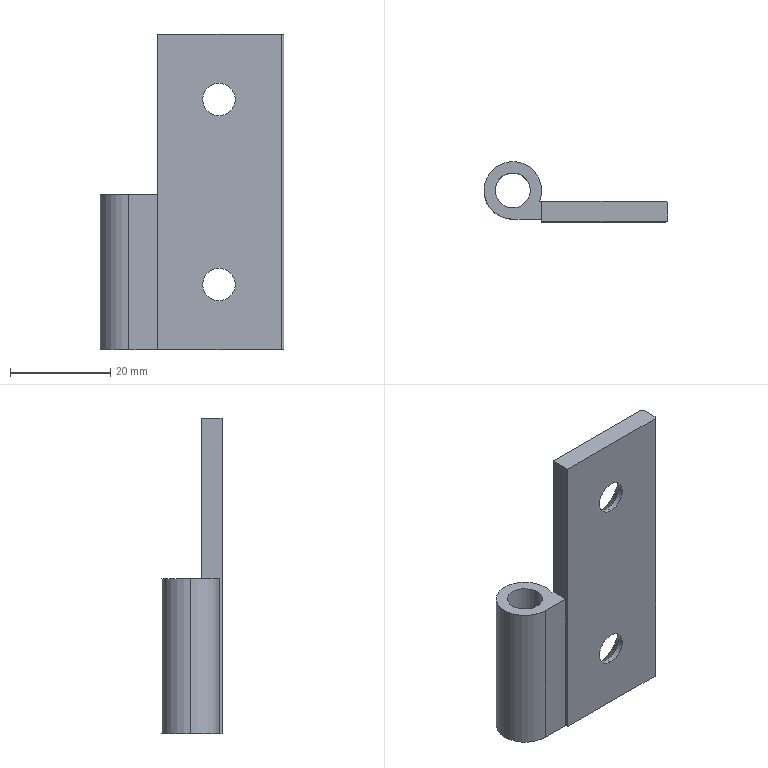Part | STEP file | _AKQ01怡合达合页2- | 1 solid | 23 faces | box 36.75 x 12.05 x 63 mm | volume 8240 mm3 | cylinder 11 | plane 8 | cone 4 | commonest cylinder face diameters 6.5 x4 11.5 x3 1 x2 7 x2
STEP:
#1=CARTESIAN_POINT('',(18.,0.,-15.25));
#2=VERTEX_POINT('',#1);
#3=CARTESIAN_POINT('',(18.,0.,-21.75));
#4=VERTEX_POINT('',#3);
#5=CARTESIAN_POINT('',(18.,0.,-18.5));
#6=DIRECTION('',(0.,-1.,0.));
#7=DIRECTION('',(0.,0.,1.));
#8=AXIS2_PLACEMENT_3D('',#5,#6,#7);
#9=CIRCLE('',#8,3.25);
#10=EDGE_CURVE('',#2,#4,#9,.T.);
#11=ORIENTED_EDGE('',*,*,#10,.T.);
#12=CARTESIAN_POINT('',(18.,1.1,-21.75));
#13=VERTEX_POINT('',#12);
#14=CARTESIAN_POINT('',(18.,0.,-21.75));
#15=DIRECTION('',(0.,1.,0.));
#16=VECTOR('',#15,1000.);
#17=LINE('',#14,#16);
#18=EDGE_CURVE('',#4,#13,#17,.T.);
#19=ORIENTED_EDGE('',*,*,#18,.T.);
#20=CARTESIAN_POINT('',(18.,1.1,-15.25));
#21=VERTEX_POINT('',#20);
#22=CARTESIAN_POINT('',(18.,1.1,-18.5));
#23=DIRECTION('',(0.,-1.,0.));
#24=DIRECTION('',(0.,0.,1.));
#25=AXIS2_PLACEMENT_3D('',#22,#23,#24);
#26=CIRCLE('',#25,3.25);
#27=EDGE_CURVE('',#21,#13,#26,.T.);
#28=ORIENTED_EDGE('',*,*,#27,.F.);
#29=CARTESIAN_POINT('',(18.,0.,-15.25));
#30=DIRECTION('',(0.,1.,0.));
#31=VECTOR('',#30,1000.);
#32=LINE('',#29,#31);
#33=EDGE_CURVE('',#2,#21,#32,.T.);
#34=ORIENTED_EDGE('',*,*,#33,.F.);
#35=EDGE_LOOP('',(#11,#19,#28,#34));
#36=FACE_OUTER_BOUND('',#35,.T.);
#37=CARTESIAN_POINT('',(18.,0.,-18.5));
#38=DIRECTION('',(0.,1.,0.));
#39=DIRECTION('',(0.,0.,1.));
#40=AXIS2_PLACEMENT_3D('',#37,#38,#39);
#41=CYLINDRICAL_SURFACE('',#40,3.25);
#42=ADVANCED_FACE('',(#36),#41,.F.);
#43=CARTESIAN_POINT('',(18.,0.,21.75));
#44=VERTEX_POINT('',#43);
#45=CARTESIAN_POINT('',(18.,0.,15.25));
#46=VERTEX_POINT('',#45);
#47=CARTESIAN_POINT('',(18.,0.,18.5));
#48=DIRECTION('',(0.,-1.,0.));
#49=DIRECTION('',(0.,0.,1.));
#50=AXIS2_PLACEMENT_3D('',#47,#48,#49);
#51=CIRCLE('',#50,3.25);
#52=EDGE_CURVE('',#44,#46,#51,.T.);
#53=ORIENTED_EDGE('',*,*,#52,.T.);
#54=CARTESIAN_POINT('',(18.,1.1,15.25));
#55=VERTEX_POINT('',#54);
#56=CARTESIAN_POINT('',(18.,0.,15.25));
#57=DIRECTION('',(0.,1.,0.));
#58=VECTOR('',#57,1000.);
#59=LINE('',#56,#58);
#60=EDGE_CURVE('',#46,#55,#59,.T.);
#61=ORIENTED_EDGE('',*,*,#60,.T.);
#62=CARTESIAN_POINT('',(18.,1.1,21.75));
#63=VERTEX_POINT('',#62);
#64=CARTESIAN_POINT('',(18.,1.1,18.5));
#65=DIRECTION('',(0.,-1.,0.));
#66=DIRECTION('',(0.,0.,1.));
#67=AXIS2_PLACEMENT_3D('',#64,#65,#66);
#68=CIRCLE('',#67,3.25);
#69=EDGE_CURVE('',#63,#55,#68,.T.);
#70=ORIENTED_EDGE('',*,*,#69,.F.);
#71=CARTESIAN_POINT('',(18.,0.,21.75));
#72=DIRECTION('',(0.,1.,0.));
#73=VECTOR('',#72,1000.);
#74=LINE('',#71,#73);
#75=EDGE_CURVE('',#44,#63,#74,.T.);
#76=ORIENTED_EDGE('',*,*,#75,.F.);
#77=EDGE_LOOP('',(#53,#61,#70,#76));
#78=FACE_OUTER_BOUND('',#77,.T.);
#79=CARTESIAN_POINT('',(18.,0.,18.5));
#80=DIRECTION('',(0.,1.,0.));
#81=DIRECTION('',(0.,0.,1.));
#82=AXIS2_PLACEMENT_3D('',#79,#80,#81);
#83=CYLINDRICAL_SURFACE('',#82,3.25);
#84=ADVANCED_FACE('',(#78),#83,.F.);
#85=CARTESIAN_POINT('',(5.75,6.3,-31.5));
#86=VERTEX_POINT('',#85);
#87=CARTESIAN_POINT('',(-5.75,6.3,-31.5));
#88=VERTEX_POINT('',#87);
#89=CARTESIAN_POINT('',(0.,6.3,-31.5));
#90=DIRECTION('',(0.,0.,1.));
#91=DIRECTION('',(1.,0.,0.));
#92=AXIS2_PLACEMENT_3D('',#89,#90,#91);
#93=CIRCLE('',#92,5.75);
#94=EDGE_CURVE('',#86,#88,#93,.T.);
#95=ORIENTED_EDGE('',*,*,#94,.T.);
#96=CARTESIAN_POINT('',(-5.75,6.3,-0.5));
#97=VERTEX_POINT('',#96);
#98=CARTESIAN_POINT('',(-5.75,6.3,31.5));
#99=DIRECTION('',(0.,0.,1.));
#100=VECTOR('',#99,1000.);
#101=LINE('',#98,#100);
#102=EDGE_CURVE('',#88,#97,#101,.T.);
#103=ORIENTED_EDGE('',*,*,#102,.T.);
#104=CARTESIAN_POINT('',(5.75,6.3,-0.5));
#105=VERTEX_POINT('',#104);
#106=CARTESIAN_POINT('',(0.,6.3,-0.5));
#107=DIRECTION('',(0.,0.,-1.));
#108=DIRECTION('',(1.,0.,0.));
#109=AXIS2_PLACEMENT_3D('',#106,#107,#108);
#110=CIRCLE('',#109,5.75);
#111=EDGE_CURVE('',#97,#105,#110,.T.);
#112=ORIENTED_EDGE('',*,*,#111,.T.);
#113=CARTESIAN_POINT('',(5.75,6.3,31.5));
#114=DIRECTION('',(0.,0.,1.));
#115=VECTOR('',#114,1000.);
#116=LINE('',#113,#115);
#117=EDGE_CURVE('',#86,#105,#116,.T.);
#118=ORIENTED_EDGE('',*,*,#117,.F.);
#119=EDGE_LOOP('',(#95,#103,#112,#118));
#120=FACE_OUTER_BOUND('',#119,.T.);
#121=CARTESIAN_POINT('',(0.,6.3,31.5));
#122=DIRECTION('',(0.,0.,1.));
#123=DIRECTION('',(1.,0.,0.));
#124=AXIS2_PLACEMENT_3D('',#121,#122,#123);
#125=CYLINDRICAL_SURFACE('',#124,5.75);
#126=ADVANCED_FACE('',(#120),#125,.T.);
#127=CARTESIAN_POINT('',(5.312,4.1,-31.5));
#128=VERTEX_POINT('',#127);
#129=CARTESIAN_POINT('',(0.,6.3,-31.5));
#130=DIRECTION('',(0.,0.,1.));
#131=DIRECTION('',(1.,0.,0.));
#132=AXIS2_PLACEMENT_3D('',#129,#130,#131);
#133=CIRCLE('',#132,5.75);
#134=EDGE_CURVE('',#128,#86,#133,.T.);
#135=ORIENTED_EDGE('',*,*,#134,.T.);
#136=ORIENTED_EDGE('',*,*,#117,.T.);
#137=CARTESIAN_POINT('',(5.312,4.1,-0.5));
#138=VERTEX_POINT('',#137);
#139=CARTESIAN_POINT('',(0.,6.3,-0.5));
#140=DIRECTION('',(0.,0.,-1.));
#141=DIRECTION('',(1.,0.,0.));
#142=AXIS2_PLACEMENT_3D('',#139,#140,#141);
#143=CIRCLE('',#142,5.75);
#144=EDGE_CURVE('',#105,#138,#143,.T.);
#145=ORIENTED_EDGE('',*,*,#144,.T.);
#146=CARTESIAN_POINT('',(5.312,4.1,31.5));
#147=DIRECTION('',(0.,0.,-1.));
#148=VECTOR('',#147,1000.);
#149=LINE('',#146,#148);
#150=EDGE_CURVE('',#138,#128,#149,.T.);
#151=ORIENTED_EDGE('',*,*,#150,.T.);
#152=EDGE_LOOP('',(#135,#136,#145,#151));
#153=FACE_OUTER_BOUND('',#152,.T.);
#154=CARTESIAN_POINT('',(0.,6.3,31.5));
#155=DIRECTION('',(0.,0.,1.));
#156=DIRECTION('',(1.,0.,0.));
#157=AXIS2_PLACEMENT_3D('',#154,#155,#156);
#158=CYLINDRICAL_SURFACE('',#157,5.75);
#159=ADVANCED_FACE('',(#153),#158,.T.);
#160=CARTESIAN_POINT('',(3.5,6.3,-31.5));
#161=VERTEX_POINT('',#160);
#162=CARTESIAN_POINT('',(-3.5,6.3,-31.5));
#163=VERTEX_POINT('',#162);
#164=CARTESIAN_POINT('',(0.,6.3,-31.5));
#165=DIRECTION('',(0.,0.,-1.));
#166=DIRECTION('',(1.,0.,0.));
#167=AXIS2_PLACEMENT_3D('',#164,#165,#166);
#168=CIRCLE('',#167,3.5);
#169=EDGE_CURVE('',#161,#163,#168,.T.);
#170=ORIENTED_EDGE('',*,*,#169,.T.);
#171=CARTESIAN_POINT('',(-3.5,6.3,-0.5));
#172=VERTEX_POINT('',#171);
#173=CARTESIAN_POINT('',(-3.5,6.3,31.5));
#174=DIRECTION('',(0.,0.,1.));
#175=VECTOR('',#174,1000.);
#176=LINE('',#173,#175);
#177=EDGE_CURVE('',#163,#172,#176,.T.);
#178=ORIENTED_EDGE('',*,*,#177,.T.);
#179=CARTESIAN_POINT('',(3.5,6.3,-0.5));
#180=VERTEX_POINT('',#179);
#181=CARTESIAN_POINT('',(0.,6.3,-0.5));
#182=DIRECTION('',(0.,0.,-1.));
#183=DIRECTION('',(1.,0.,0.));
#184=AXIS2_PLACEMENT_3D('',#181,#182,#183);
#185=CIRCLE('',#184,3.5);
#186=EDGE_CURVE('',#180,#172,#185,.T.);
#187=ORIENTED_EDGE('',*,*,#186,.F.);
#188=CARTESIAN_POINT('',(3.5,6.3,31.5));
#189=DIRECTION('',(0.,0.,1.));
#190=VECTOR('',#189,1000.);
#191=LINE('',#188,#190);
#192=EDGE_CURVE('',#161,#180,#191,.T.);
#193=ORIENTED_EDGE('',*,*,#192,.F.);
#194=EDGE_LOOP('',(#170,#178,#187,#193));
#195=FACE_OUTER_BOUND('',#194,.T.);
#196=CARTESIAN_POINT('',(0.,6.3,31.5));
#197=DIRECTION('',(0.,0.,1.));
#198=DIRECTION('',(1.,0.,0.));
#199=AXIS2_PLACEMENT_3D('',#196,#197,#198);
#200=CYLINDRICAL_SURFACE('',#199,3.5);
#201=ADVANCED_FACE('',(#195),#200,.F.);
#202=ORIENTED_EDGE('',*,*,#27,.T.);
#203=CARTESIAN_POINT('',(18.,4.1,-24.75));
#204=VERTEX_POINT('',#203);
#205=CARTESIAN_POINT('',(18.,4.1,-24.75));
#206=DIRECTION('',(0.,0.7071,-0.7071));
#207=VECTOR('',#206,1000.);
#208=LINE('',#205,#207);
#209=EDGE_CURVE('',#13,#204,#208,.T.);
#210=ORIENTED_EDGE('',*,*,#209,.T.);
#211=CARTESIAN_POINT('',(18.,4.1,-12.25));
#212=VERTEX_POINT('',#211);
#213=CARTESIAN_POINT('',(18.,4.1,-18.5));
#214=DIRECTION('',(0.,1.,0.));
#215=DIRECTION('',(0.,0.,1.));
#216=AXIS2_PLACEMENT_3D('',#213,#214,#215);
#217=CIRCLE('',#216,6.25);
#218=EDGE_CURVE('',#204,#212,#217,.T.);
#219=ORIENTED_EDGE('',*,*,#218,.T.);
#220=CARTESIAN_POINT('',(18.,4.1,-12.25));
#221=DIRECTION('',(0.,0.7071,0.7071));
#222=VECTOR('',#221,1000.);
#223=LINE('',#220,#222);
#224=EDGE_CURVE('',#21,#212,#223,.T.);
#225=ORIENTED_EDGE('',*,*,#224,.F.);
#226=EDGE_LOOP('',(#202,#210,#219,#225));
#227=FACE_OUTER_BOUND('',#226,.T.);
#228=CARTESIAN_POINT('',(18.,4.1,-18.5));
#229=DIRECTION('',(0.,1.,0.));
#230=DIRECTION('',(0.,0.,1.));
#231=AXIS2_PLACEMENT_3D('',#228,#229,#230);
#232=CONICAL_SURFACE('',#231,6.25,0.7854);
#233=ADVANCED_FACE('',(#227),#232,.F.);
#234=ORIENTED_EDGE('',*,*,#69,.T.);
#235=CARTESIAN_POINT('',(18.,4.1,12.25));
#236=VERTEX_POINT('',#235);
#237=CARTESIAN_POINT('',(18.,4.1,12.25));
#238=DIRECTION('',(0.,0.7071,-0.7071));
#239=VECTOR('',#238,1000.);
#240=LINE('',#237,#239);
#241=EDGE_CURVE('',#55,#236,#240,.T.);
#242=ORIENTED_EDGE('',*,*,#241,.T.);
#243=CARTESIAN_POINT('',(18.,4.1,24.75));
#244=VERTEX_POINT('',#243);
#245=CARTESIAN_POINT('',(18.,4.1,18.5));
#246=DIRECTION('',(0.,1.,0.));
#247=DIRECTION('',(0.,0.,1.));
#248=AXIS2_PLACEMENT_3D('',#245,#246,#247);
#249=CIRCLE('',#248,6.25);
#250=EDGE_CURVE('',#236,#244,#249,.T.);
#251=ORIENTED_EDGE('',*,*,#250,.T.);
#252=CARTESIAN_POINT('',(18.,4.1,24.75));
#253=DIRECTION('',(0.,0.7071,0.7071));
#254=VECTOR('',#253,1000.);
#255=LINE('',#252,#254);
#256=EDGE_CURVE('',#63,#244,#255,.T.);
#257=ORIENTED_EDGE('',*,*,#256,.F.);
#258=EDGE_LOOP('',(#234,#242,#251,#257));
#259=FACE_OUTER_BOUND('',#258,.T.);
#260=CARTESIAN_POINT('',(18.,4.1,18.5));
#261=DIRECTION('',(0.,1.,0.));
#262=DIRECTION('',(0.,0.,1.));
#263=AXIS2_PLACEMENT_3D('',#260,#261,#262);
#264=CONICAL_SURFACE('',#263,6.25,0.7854);
#265=ADVANCED_FACE('',(#259),#264,.F.);
#266=CARTESIAN_POINT('',(30.5,0.,31.5));
#267=VERTEX_POINT('',#266);
#268=CARTESIAN_POINT('',(30.5,0.,-31.5));
#269=VERTEX_POINT('',#268);
#270=CARTESIAN_POINT('',(30.5,0.,31.5));
#271=DIRECTION('',(0.,0.,-1.));
#272=VECTOR('',#271,1000.);
#273=LINE('',#270,#272);
#274=EDGE_CURVE('',#267,#269,#273,.T.);
#275=ORIENTED_EDGE('',*,*,#274,.F.);
#276=CARTESIAN_POINT('',(5.75,0.,31.5));
#277=VERTEX_POINT('',#276);
#278=CARTESIAN_POINT('',(5.75,0.,31.5));
#279=DIRECTION('',(1.,0.,0.));
#280=VECTOR('',#279,1000.);
#281=LINE('',#278,#280);
#282=EDGE_CURVE('',#277,#267,#281,.T.);
#283=ORIENTED_EDGE('',*,*,#282,.F.);
#284=CARTESIAN_POINT('',(5.75,0.,-31.5));
#285=VERTEX_POINT('',#284);
#286=CARTESIAN_POINT('',(5.75,0.,31.5));
#287=DIRECTION('',(0.,0.,1.));
#288=VECTOR('',#287,1000.);
#289=LINE('',#286,#288);
#290=EDGE_CURVE('',#285,#277,#289,.T.);
#291=ORIENTED_EDGE('',*,*,#290,.F.);
#292=CARTESIAN_POINT('',(5.75,0.,-31.5));
#293=DIRECTION('',(-1.,0.,0.));
#294=VECTOR('',#293,1000.);
#295=LINE('',#292,#294);
#296=EDGE_CURVE('',#269,#285,#295,.T.);
#297=ORIENTED_EDGE('',*,*,#296,.F.);
#298=EDGE_LOOP('',(#275,#283,#291,#297));
#299=FACE_OUTER_BOUND('',#298,.T.);
#300=ORIENTED_EDGE('',*,*,#10,.F.);
#301=CARTESIAN_POINT('',(18.,0.,-18.5));
#302=DIRECTION('',(0.,-1.,0.));
#303=DIRECTION('',(0.,0.,1.));
#304=AXIS2_PLACEMENT_3D('',#301,#302,#303);
#305=CIRCLE('',#304,3.25);
#306=EDGE_CURVE('',#4,#2,#305,.T.);
#307=ORIENTED_EDGE('',*,*,#306,.F.);
#308=EDGE_LOOP('',(#300,#307));
#309=FACE_BOUND('',#308,.T.);
#310=ORIENTED_EDGE('',*,*,#52,.F.);
#311=CARTESIAN_POINT('',(18.,0.,18.5));
#312=DIRECTION('',(0.,-1.,0.));
#313=DIRECTION('',(0.,0.,1.));
#314=AXIS2_PLACEMENT_3D('',#311,#312,#313);
#315=CIRCLE('',#314,3.25);
#316=EDGE_CURVE('',#46,#44,#315,.T.);
#317=ORIENTED_EDGE('',*,*,#316,.F.);
#318=EDGE_LOOP('',(#310,#317));
#319=FACE_BOUND('',#318,.T.);
#320=CARTESIAN_POINT('',(5.75,0.,31.5));
#321=DIRECTION('',(0.,1.,0.));
#322=DIRECTION('',(0.,0.,1.));
#323=AXIS2_PLACEMENT_3D('',#320,#321,#322);
#324=PLANE('',#323);
#325=ADVANCED_FACE('',(#299,#309,#319),#324,.F.);
#326=CARTESIAN_POINT('',(31.,3.6,-31.5));
#327=VERTEX_POINT('',#326);
#328=CARTESIAN_POINT('',(30.5,4.1,-31.5));
#329=VERTEX_POINT('',#328);
#330=CARTESIAN_POINT('',(30.5,3.6,-31.5));
#331=DIRECTION('',(0.,0.,1.));
#332=DIRECTION('',(1.,0.,0.));
#333=AXIS2_PLACEMENT_3D('',#330,#331,#332);
#334=CIRCLE('',#333,0.5);
#335=EDGE_CURVE('',#327,#329,#334,.T.);
#336=ORIENTED_EDGE('',*,*,#335,.F.);
#337=CARTESIAN_POINT('',(31.,0.5,-31.5));
#338=VERTEX_POINT('',#337);
#339=CARTESIAN_POINT('',(31.,6.3,-31.5));
#340=DIRECTION('',(0.,1.,0.));
#341=VECTOR('',#340,1000.);
#342=LINE('',#339,#341);
#343=EDGE_CURVE('',#338,#327,#342,.T.);
#344=ORIENTED_EDGE('',*,*,#343,.F.);
#345=CARTESIAN_POINT('',(30.5,0.5,-31.5));
#346=DIRECTION('',(0.,0.,1.));
#347=DIRECTION('',(1.,0.,0.));
#348=AXIS2_PLACEMENT_3D('',#345,#346,#347);
#349=CIRCLE('',#348,0.5);
#350=EDGE_CURVE('',#269,#338,#349,.T.);
#351=ORIENTED_EDGE('',*,*,#350,.F.);
#352=ORIENTED_EDGE('',*,*,#296,.T.);
#353=CARTESIAN_POINT('',(5.75,0.55,-31.5));
#354=VERTEX_POINT('',#353);
#355=CARTESIAN_POINT('',(5.75,6.3,-31.5));
#356=DIRECTION('',(0.,-1.,0.));
#357=VECTOR('',#356,1000.);
#358=LINE('',#355,#357);
#359=EDGE_CURVE('',#354,#285,#358,.T.);
#360=ORIENTED_EDGE('',*,*,#359,.F.);
#361=CARTESIAN_POINT('',(0.,0.55,-31.5));
#362=VERTEX_POINT('',#361);
#363=CARTESIAN_POINT('',(0.,0.55,-31.5));
#364=DIRECTION('',(1.,0.,0.));
#365=VECTOR('',#364,1000.);
#366=LINE('',#363,#365);
#367=EDGE_CURVE('',#362,#354,#366,.T.);
#368=ORIENTED_EDGE('',*,*,#367,.F.);
#369=CARTESIAN_POINT('',(0.,6.3,-31.5));
#370=DIRECTION('',(0.,0.,1.));
#371=DIRECTION('',(1.,0.,0.));
#372=AXIS2_PLACEMENT_3D('',#369,#370,#371);
#373=CIRCLE('',#372,5.75);
#374=EDGE_CURVE('',#88,#362,#373,.T.);
#375=ORIENTED_EDGE('',*,*,#374,.F.);
#376=ORIENTED_EDGE('',*,*,#94,.F.);
#377=ORIENTED_EDGE('',*,*,#134,.F.);
#378=CARTESIAN_POINT('',(0.,4.1,-31.5));
#379=DIRECTION('',(-1.,0.,0.));
#380=VECTOR('',#379,1000.);
#381=LINE('',#378,#380);
#382=EDGE_CURVE('',#329,#128,#381,.T.);
#383=ORIENTED_EDGE('',*,*,#382,.F.);
#384=EDGE_LOOP('',(#336,#344,#351,#352,#360,#368,#375,#376,#377,#383));
#385=FACE_OUTER_BOUND('',#384,.T.);
#386=ORIENTED_EDGE('',*,*,#169,.F.);
#387=CARTESIAN_POINT('',(0.,6.3,-31.5));
#388=DIRECTION('',(0.,0.,-1.));
#389=DIRECTION('',(1.,0.,0.));
#390=AXIS2_PLACEMENT_3D('',#387,#388,#389);
#391=CIRCLE('',#390,3.5);
#392=EDGE_CURVE('',#163,#161,#391,.T.);
#393=ORIENTED_EDGE('',*,*,#392,.F.);
#394=EDGE_LOOP('',(#386,#393));
#395=FACE_BOUND('',#394,.T.);
#396=CARTESIAN_POINT('',(0.,6.3,-31.5));
#397=DIRECTION('',(0.,0.,1.));
#398=DIRECTION('',(1.,0.,0.));
#399=AXIS2_PLACEMENT_3D('',#396,#397,#398);
#400=PLANE('',#399);
#401=ADVANCED_FACE('',(#385,#395),#400,.F.);
#402=CARTESIAN_POINT('',(31.,0.5,31.5));
#403=VERTEX_POINT('',#402);
#404=CARTESIAN_POINT('',(30.5,0.5,31.5));
#405=DIRECTION('',(0.,0.,-1.));
#406=DIRECTION('',(1.,0.,0.));
#407=AXIS2_PLACEMENT_3D('',#404,#405,#406);
#408=CIRCLE('',#407,0.5);
#409=EDGE_CURVE('',#403,#267,#408,.T.);
#410=ORIENTED_EDGE('',*,*,#409,.T.);
#411=ORIENTED_EDGE('',*,*,#274,.T.);
#412=ORIENTED_EDGE('',*,*,#350,.T.);
#413=CARTESIAN_POINT('',(31.,0.5,31.5));
#414=DIRECTION('',(0.,0.,1.));
#415=VECTOR('',#414,1000.);
#416=LINE('',#413,#415);
#417=EDGE_CURVE('',#338,#403,#416,.T.);
#418=ORIENTED_EDGE('',*,*,#417,.T.);
#419=EDGE_LOOP('',(#410,#411,#412,#418));
#420=FACE_OUTER_BOUND('',#419,.T.);
#421=CARTESIAN_POINT('',(30.5,0.5,31.5));
#422=DIRECTION('',(0.,0.,1.));
#423=DIRECTION('',(1.,0.,0.));
#424=AXIS2_PLACEMENT_3D('',#421,#422,#423);
#425=CYLINDRICAL_SURFACE('',#424,0.5);
#426=ADVANCED_FACE('',(#420),#425,.T.);
#427=CARTESIAN_POINT('',(31.,3.6,31.5));
#428=VERTEX_POINT('',#427);
#429=CARTESIAN_POINT('',(31.,6.3,31.5));
#430=DIRECTION('',(0.,1.,0.));
#431=VECTOR('',#430,1000.);
#432=LINE('',#429,#431);
#433=EDGE_CURVE('',#403,#428,#432,.T.);
#434=ORIENTED_EDGE('',*,*,#433,.T.);
#435=CARTESIAN_POINT('',(30.5,4.1,31.5));
#436=VERTEX_POINT('',#435);
#437=CARTESIAN_POINT('',(30.5,3.6,31.5));
#438=DIRECTION('',(0.,0.,-1.));
#439=DIRECTION('',(1.,0.,0.));
#440=AXIS2_PLACEMENT_3D('',#437,#438,#439);
#441=CIRCLE('',#440,0.5);
#442=EDGE_CURVE('',#436,#428,#441,.T.);
#443=ORIENTED_EDGE('',*,*,#442,.F.);
#444=CARTESIAN_POINT('',(5.75,4.1,31.5));
#445=VERTEX_POINT('',#444);
#446=CARTESIAN_POINT('',(0.,4.1,31.5));
#447=DIRECTION('',(-1.,0.,0.));
#448=VECTOR('',#447,1000.);
#449=LINE('',#446,#448);
#450=EDGE_CURVE('',#436,#445,#449,.T.);
#451=ORIENTED_EDGE('',*,*,#450,.T.);
#452=CARTESIAN_POINT('',(5.75,6.3,31.5));
#453=DIRECTION('',(0.,-1.,0.));
#454=VECTOR('',#453,1000.);
#455=LINE('',#452,#454);
#456=EDGE_CURVE('',#445,#277,#455,.T.);
#457=ORIENTED_EDGE('',*,*,#456,.T.);
#458=ORIENTED_EDGE('',*,*,#282,.T.);
#459=ORIENTED_EDGE('',*,*,#409,.F.);
#460=EDGE_LOOP('',(#434,#443,#451,#457,#458,#459));
#461=FACE_OUTER_BOUND('',#460,.T.);
#462=CARTESIAN_POINT('',(0.,6.3,31.5));
#463=DIRECTION('',(0.,0.,1.));
#464=DIRECTION('',(1.,0.,0.));
#465=AXIS2_PLACEMENT_3D('',#462,#463,#464);
#466=PLANE('',#465);
#467=ADVANCED_FACE('',(#461),#466,.T.);
#468=CARTESIAN_POINT('',(5.75,4.1,-0.5));
#469=VERTEX_POINT('',#468);
#470=CARTESIAN_POINT('',(5.75,4.1,31.5));
#471=DIRECTION('',(0.,0.,1.));
#472=VECTOR('',#471,1000.);
#473=LINE('',#470,#472);
#474=EDGE_CURVE('',#469,#445,#473,.T.);
#475=ORIENTED_EDGE('',*,*,#474,.F.);
#476=CARTESIAN_POINT('',(5.75,0.55,-0.5));
#477=VERTEX_POINT('',#476);
#478=CARTESIAN_POINT('',(5.75,0.55,-0.5));
#479=DIRECTION('',(0.,1.,0.));
#480=VECTOR('',#479,1000.);
#481=LINE('',#478,#480);
#482=EDGE_CURVE('',#477,#469,#481,.T.);
#483=ORIENTED_EDGE('',*,*,#482,.F.);
#484=CARTESIAN_POINT('',(5.75,0.55,31.5));
#485=DIRECTION('',(0.,0.,1.));
#486=VECTOR('',#485,1000.);
#487=LINE('',#484,#486);
#488=EDGE_CURVE('',#354,#477,#487,.T.);
#489=ORIENTED_EDGE('',*,*,#488,.F.);
#490=ORIENTED_EDGE('',*,*,#359,.T.);
#491=ORIENTED_EDGE('',*,*,#290,.T.);
#492=ORIENTED_EDGE('',*,*,#456,.F.);
#493=EDGE_LOOP('',(#475,#483,#489,#490,#491,#492));
#494=FACE_OUTER_BOUND('',#493,.T.);
#495=CARTESIAN_POINT('',(5.75,0.55,31.5));
#496=DIRECTION('',(1.,0.,0.));
#497=DIRECTION('',(0.,1.,0.));
#498=AXIS2_PLACEMENT_3D('',#495,#496,#497);
#499=PLANE('',#498);
#500=ADVANCED_FACE('',(#494),#499,.F.);
#501=ORIENTED_EDGE('',*,*,#18,.F.);
#502=ORIENTED_EDGE('',*,*,#306,.T.);
#503=ORIENTED_EDGE('',*,*,#33,.T.);
#504=CARTESIAN_POINT('',(18.,1.1,-18.5));
#505=DIRECTION('',(0.,-1.,0.));
#506=DIRECTION('',(0.,0.,1.));
#507=AXIS2_PLACEMENT_3D('',#504,#505,#506);
#508=CIRCLE('',#507,3.25);
#509=EDGE_CURVE('',#13,#21,#508,.T.);
#510=ORIENTED_EDGE('',*,*,#509,.F.);
#511=EDGE_LOOP('',(#501,#502,#503,#510));
#512=FACE_OUTER_BOUND('',#511,.T.);
#513=CARTESIAN_POINT('',(18.,0.,-18.5));
#514=DIRECTION('',(0.,1.,0.));
#515=DIRECTION('',(0.,0.,1.));
#516=AXIS2_PLACEMENT_3D('',#513,#514,#515);
#517=CYLINDRICAL_SURFACE('',#516,3.25);
#518=ADVANCED_FACE('',(#512),#517,.F.);
#519=ORIENTED_EDGE('',*,*,#60,.F.);
#520=ORIENTED_EDGE('',*,*,#316,.T.);
#521=ORIENTED_EDGE('',*,*,#75,.T.);
#522=CARTESIAN_POINT('',(18.,1.1,18.5));
#523=DIRECTION('',(0.,-1.,0.));
#524=DIRECTION('',(0.,0.,1.));
#525=AXIS2_PLACEMENT_3D('',#522,#523,#524);
#526=CIRCLE('',#525,3.25);
#527=EDGE_CURVE('',#55,#63,#526,.T.);
#528=ORIENTED_EDGE('',*,*,#527,.F.);
#529=EDGE_LOOP('',(#519,#520,#521,#528));
#530=FACE_OUTER_BOUND('',#529,.T.);
#531=CARTESIAN_POINT('',(18.,0.,18.5));
#532=DIRECTION('',(0.,1.,0.));
#533=DIRECTION('',(0.,0.,1.));
#534=AXIS2_PLACEMENT_3D('',#531,#532,#533);
#535=CYLINDRICAL_SURFACE('',#534,3.25);
#536=ADVANCED_FACE('',(#530),#535,.F.);
#537=ORIENTED_EDGE('',*,*,#450,.F.);
#538=CARTESIAN_POINT('',(30.5,4.1,31.5));
#539=DIRECTION('',(0.,0.,1.));
#540=VECTOR('',#539,1000.);
#541=LINE('',#538,#540);
#542=EDGE_CURVE('',#329,#436,#541,.T.);
#543=ORIENTED_EDGE('',*,*,#542,.F.);
#544=ORIENTED_EDGE('',*,*,#382,.T.);
#545=ORIENTED_EDGE('',*,*,#150,.F.);
#546=CARTESIAN_POINT('',(30.5,4.1,-0.5));
#547=DIRECTION('',(-1.,0.,0.));
#548=VECTOR('',#547,1000.);
#549=LINE('',#546,#548);
#550=EDGE_CURVE('',#469,#138,#549,.T.);
#551=ORIENTED_EDGE('',*,*,#550,.F.);
#552=ORIENTED_EDGE('',*,*,#474,.T.);
#553=EDGE_LOOP('',(#537,#543,#544,#545,#551,#552));
#554=FACE_OUTER_BOUND('',#553,.T.);
#555=CARTESIAN_POINT('',(18.,4.1,-18.5));
#556=DIRECTION('',(0.,1.,0.));
#557=DIRECTION('',(0.,0.,1.));
#558=AXIS2_PLACEMENT_3D('',#555,#556,#557);
#559=CIRCLE('',#558,6.25);
#560=EDGE_CURVE('',#212,#204,#559,.T.);
#561=ORIENTED_EDGE('',*,*,#560,.F.);
#562=ORIENTED_EDGE('',*,*,#218,.F.);
#563=EDGE_LOOP('',(#561,#562));
#564=FACE_BOUND('',#563,.T.);
#565=CARTESIAN_POINT('',(18.,4.1,18.5));
#566=DIRECTION('',(0.,1.,0.));
#567=DIRECTION('',(0.,0.,1.));
#568=AXIS2_PLACEMENT_3D('',#565,#566,#567);
#569=CIRCLE('',#568,6.25);
#570=EDGE_CURVE('',#244,#236,#569,.T.);
#571=ORIENTED_EDGE('',*,*,#570,.F.);
#572=ORIENTED_EDGE('',*,*,#250,.F.);
#573=EDGE_LOOP('',(#571,#572));
#574=FACE_BOUND('',#573,.T.);
#575=CARTESIAN_POINT('',(30.5,4.1,31.5));
#576=DIRECTION('',(0.,-1.,0.));
#577=DIRECTION('',(0.,0.,-1.));
#578=AXIS2_PLACEMENT_3D('',#575,#576,#577);
#579=PLANE('',#578);
#580=ADVANCED_FACE('',(#554,#564,#574),#579,.F.);
#581=CARTESIAN_POINT('',(31.,3.6,31.5));
#582=DIRECTION('',(0.,0.,-1.));
#583=VECTOR('',#582,1000.);
#584=LINE('',#581,#583);
#585=EDGE_CURVE('',#428,#327,#584,.T.);
#586=ORIENTED_EDGE('',*,*,#585,.F.);
#587=ORIENTED_EDGE('',*,*,#433,.F.);
#588=ORIENTED_EDGE('',*,*,#417,.F.);
#589=ORIENTED_EDGE('',*,*,#343,.T.);
#590=EDGE_LOOP('',(#586,#587,#588,#589));
#591=FACE_OUTER_BOUND('',#590,.T.);
#592=CARTESIAN_POINT('',(31.,0.5,31.5));
#593=DIRECTION('',(-1.,0.,0.));
#594=DIRECTION('',(0.,0.,1.));
#595=AXIS2_PLACEMENT_3D('',#592,#593,#594);
#596=PLANE('',#595);
#597=ADVANCED_FACE('',(#591),#596,.F.);
#598=CARTESIAN_POINT('',(0.,0.55,-0.5));
#599=VERTEX_POINT('',#598);
#600=CARTESIAN_POINT('',(0.,0.55,31.5));
#601=DIRECTION('',(0.,0.,1.));
#602=VECTOR('',#601,1000.);
#603=LINE('',#600,#602);
#604=EDGE_CURVE('',#362,#599,#603,.T.);
#605=ORIENTED_EDGE('',*,*,#604,.F.);
#606=ORIENTED_EDGE('',*,*,#367,.T.);
#607=ORIENTED_EDGE('',*,*,#488,.T.);
#608=CARTESIAN_POINT('',(0.,0.55,-0.5));
#609=DIRECTION('',(1.,0.,0.));
#610=VECTOR('',#609,1000.);
#611=LINE('',#608,#610);
#612=EDGE_CURVE('',#599,#477,#611,.T.);
#613=ORIENTED_EDGE('',*,*,#612,.F.);
#614=EDGE_LOOP('',(#605,#606,#607,#613));
#615=FACE_OUTER_BOUND('',#614,.T.);
#616=CARTESIAN_POINT('',(0.,0.55,31.5));
#617=DIRECTION('',(0.,1.,0.));
#618=DIRECTION('',(0.,0.,1.));
#619=AXIS2_PLACEMENT_3D('',#616,#617,#618);
#620=PLANE('',#619);
#621=ADVANCED_FACE('',(#615),#620,.F.);
#622=ORIENTED_EDGE('',*,*,#102,.F.);
#623=ORIENTED_EDGE('',*,*,#374,.T.);
#624=ORIENTED_EDGE('',*,*,#604,.T.);
#625=CARTESIAN_POINT('',(0.,6.3,-0.5));
#626=DIRECTION('',(0.,0.,-1.));
#627=DIRECTION('',(1.,0.,0.));
#628=AXIS2_PLACEMENT_3D('',#625,#626,#627);
#629=CIRCLE('',#628,5.75);
#630=EDGE_CURVE('',#599,#97,#629,.T.);
#631=ORIENTED_EDGE('',*,*,#630,.T.);
#632=EDGE_LOOP('',(#622,#623,#624,#631));
#633=FACE_OUTER_BOUND('',#632,.T.);
#634=CARTESIAN_POINT('',(0.,6.3,31.5));
#635=DIRECTION('',(0.,0.,1.));
#636=DIRECTION('',(1.,0.,0.));
#637=AXIS2_PLACEMENT_3D('',#634,#635,#636);
#638=CYLINDRICAL_SURFACE('',#637,5.75);
#639=ADVANCED_FACE('',(#633),#638,.T.);
#640=ORIENTED_EDGE('',*,*,#177,.F.);
#641=ORIENTED_EDGE('',*,*,#392,.T.);
#642=ORIENTED_EDGE('',*,*,#192,.T.);
#643=CARTESIAN_POINT('',(0.,6.3,-0.5));
#644=DIRECTION('',(0.,0.,-1.));
#645=DIRECTION('',(1.,0.,0.));
#646=AXIS2_PLACEMENT_3D('',#643,#644,#645);
#647=CIRCLE('',#646,3.5);
#648=EDGE_CURVE('',#172,#180,#647,.T.);
#649=ORIENTED_EDGE('',*,*,#648,.F.);
#650=EDGE_LOOP('',(#640,#641,#642,#649));
#651=FACE_OUTER_BOUND('',#650,.T.);
#652=CARTESIAN_POINT('',(0.,6.3,31.5));
#653=DIRECTION('',(0.,0.,1.));
#654=DIRECTION('',(1.,0.,0.));
#655=AXIS2_PLACEMENT_3D('',#652,#653,#654);
#656=CYLINDRICAL_SURFACE('',#655,3.5);
#657=ADVANCED_FACE('',(#651),#656,.F.);
#658=ORIENTED_EDGE('',*,*,#612,.T.);
#659=ORIENTED_EDGE('',*,*,#482,.T.);
#660=ORIENTED_EDGE('',*,*,#550,.T.);
#661=ORIENTED_EDGE('',*,*,#144,.F.);
#662=ORIENTED_EDGE('',*,*,#111,.F.);
#663=ORIENTED_EDGE('',*,*,#630,.F.);
#664=EDGE_LOOP('',(#658,#659,#660,#661,#662,#663));
#665=FACE_OUTER_BOUND('',#664,.T.);
#666=ORIENTED_EDGE('',*,*,#186,.T.);
#667=ORIENTED_EDGE('',*,*,#648,.T.);
#668=EDGE_LOOP('',(#666,#667));
#669=FACE_BOUND('',#668,.T.);
#670=CARTESIAN_POINT('',(5.75,25.4,-0.5));
#671=DIRECTION('',(0.,0.,1.));
#672=DIRECTION('',(1.,0.,0.));
#673=AXIS2_PLACEMENT_3D('',#670,#671,#672);
#674=PLANE('',#673);
#675=ADVANCED_FACE('',(#665,#669),#674,.T.);
#676=ORIENTED_EDGE('',*,*,#209,.F.);
#677=ORIENTED_EDGE('',*,*,#509,.T.);
#678=ORIENTED_EDGE('',*,*,#224,.T.);
#679=ORIENTED_EDGE('',*,*,#560,.T.);
#680=EDGE_LOOP('',(#676,#677,#678,#679));
#681=FACE_OUTER_BOUND('',#680,.T.);
#682=CARTESIAN_POINT('',(18.,4.1,-18.5));
#683=DIRECTION('',(0.,1.,0.));
#684=DIRECTION('',(0.,0.,1.));
#685=AXIS2_PLACEMENT_3D('',#682,#683,#684);
#686=CONICAL_SURFACE('',#685,6.25,0.7854);
#687=ADVANCED_FACE('',(#681),#686,.F.);
#688=ORIENTED_EDGE('',*,*,#241,.F.);
#689=ORIENTED_EDGE('',*,*,#527,.T.);
#690=ORIENTED_EDGE('',*,*,#256,.T.);
#691=ORIENTED_EDGE('',*,*,#570,.T.);
#692=EDGE_LOOP('',(#688,#689,#690,#691));
#693=FACE_OUTER_BOUND('',#692,.T.);
#694=CARTESIAN_POINT('',(18.,4.1,18.5));
#695=DIRECTION('',(0.,1.,0.));
#696=DIRECTION('',(0.,0.,1.));
#697=AXIS2_PLACEMENT_3D('',#694,#695,#696);
#698=CONICAL_SURFACE('',#697,6.25,0.7854);
#699=ADVANCED_FACE('',(#693),#698,.F.);
#700=ORIENTED_EDGE('',*,*,#442,.T.);
#701=ORIENTED_EDGE('',*,*,#585,.T.);
#702=ORIENTED_EDGE('',*,*,#335,.T.);
#703=ORIENTED_EDGE('',*,*,#542,.T.);
#704=EDGE_LOOP('',(#700,#701,#702,#703));
#705=FACE_OUTER_BOUND('',#704,.T.);
#706=CARTESIAN_POINT('',(30.5,3.6,31.5));
#707=DIRECTION('',(0.,0.,1.));
#708=DIRECTION('',(1.,0.,0.));
#709=AXIS2_PLACEMENT_3D('',#706,#707,#708);
#710=CYLINDRICAL_SURFACE('',#709,0.5);
#711=ADVANCED_FACE('',(#705),#710,.T.);
#712=CLOSED_SHELL('',(#42,#84,#126,#159,#201,#233,#265,#325,#401,#426,#467,#500,#518,#536,#580,#597,#621,#639,#657,#675,#687,#699,#711));
#713=MANIFOLD_SOLID_BREP('',#712);
#714=CARTESIAN_POINT('',(0.,0.,0.));
#715=DIRECTION('',(0.,0.,1.));
#716=DIRECTION('',(1.,0.,0.));
#717=AXIS2_PLACEMENT_3D('',#714,#715,#716);
#718=(LENGTH_UNIT()NAMED_UNIT(*)SI_UNIT(.MILLI.,.METRE.));
#719=UNCERTAINTY_MEASURE_WITH_UNIT(LENGTH_MEASURE(0.00001),#718,'','');
#720=(NAMED_UNIT(*)PLANE_ANGLE_UNIT()SI_UNIT($,.RADIAN.));
#721=(NAMED_UNIT(*)SI_UNIT($,.STERADIAN.)SOLID_ANGLE_UNIT());
#722=(GEOMETRIC_REPRESENTATION_CONTEXT(3)GLOBAL_UNCERTAINTY_ASSIGNED_CONTEXT((#719))GLOBAL_UNIT_ASSIGNED_CONTEXT((#718,#720,#721))REPRESENTATION_CONTEXT('',''));
#723=ADVANCED_BREP_SHAPE_REPRESENTATION('',(#713,#717),#722);